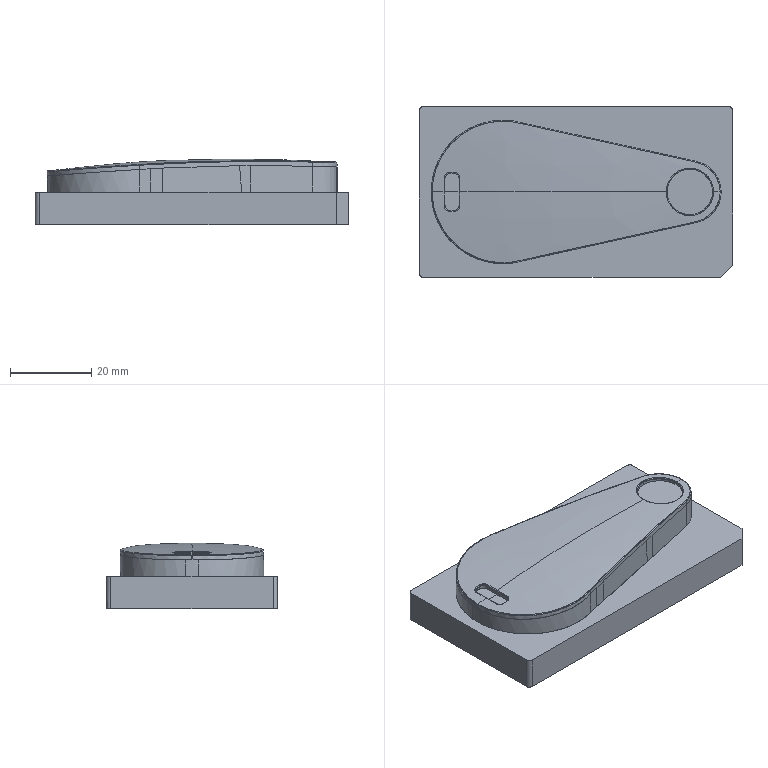NC program | PowerMill | posted with a generic post | part box 77 x 42 x 16.114 mm
Lines 17578 to 18293 of 134652:
N17675 M6
N17676 S18000 M03
N17677 G00 G90 X0.0 Y0.0
N17678 G43 Z10.803 H7
N17679
N17680 G05 P10000 R8
N17681 X35.0974 Y-6.155
N17682 Z-1.4614
N17683 G01 Z-2.6614 F1200.0
N17684 X35.0633 Y-6.1892 Z-2.6414 F2000.0
N17685 X35.0136 Y-6.2388 Z-2.6177
N17686 X34.9538 Y-6.2987 Z-2.5949
N17687 X34.8809 Y-6.3715 Z-2.5733
N17688 X34.7915 Y-6.4609 Z-2.5538
N17689 X34.711 Y-6.5414 Z-2.5419
N17690 X34.6456 Y-6.6069 Z-2.5361
N17691 X34.5916 Y-6.6609 Z-2.5342
N17692 X34.5388 Y-6.7136 Z-2.5355
N17693 X34.482 Y-6.7704 Z-2.5401
N17694 X34.388 Y-6.8644 Z-2.5527
N17695 X34.3036 Y-6.9488 Z-2.5709
N17696 X34.2267 Y-7.0258 Z-2.5946
N17697 X34.1559 Y-7.0966 Z-2.6239
N17698 X34.0903 Y-7.1621 Z-2.6586
N17699 X34.029 Y-7.2234 Z-2.6992
N17700 X33.6957 Y-7.4719 Z-2.6101
N17701 X33.7483 Y-7.4193 Z-2.5656
N17702 X33.8073 Y-7.3602 Z-2.5243
N17703 X33.8738 Y-7.2938 Z-2.4858
N17704 X33.9483 Y-7.2193 Z-2.4504
N17705 X34.0316 Y-7.136 Z-2.4185
N17706 X34.1246 Y-7.043 Z-2.3906
N17707 X34.2271 Y-6.9405 Z-2.3677
N17708 X34.3349 Y-6.8327 Z-2.3511
N17709 X34.4335 Y-6.734 Z-2.3421
N17710 X34.5208 Y-6.6468 Z-2.3389
N17711 X34.5972 Y-6.5704 Z-2.3399
N17712 X34.6638 Y-6.5038 Z-2.3437
N17713 X34.7235 Y-6.4441 Z-2.35
N17714 X34.8002 Y-6.3674 Z-2.3616
N17715 X34.8886 Y-6.2789 Z-2.379
N17716 X34.9883 Y-6.1793 Z-2.4046
N17717 X35.0858 Y-6.0818 Z-2.4365
N17718 X35.1732 Y-5.9944 Z-2.4723
N17719 X35.2506 Y-5.917 Z-2.5109
N17720 X35.3188 Y-5.8487 Z-2.552
N17721 X35.379 Y-5.7886 Z-2.5954
N17722 X35.4317 Y-5.7358 Z-2.6411
N17723 X35.4585 Y-5.7091 Z-2.6679
N17724 X35.7163 Y-5.3665 Z-2.7108
N17725 X35.6786 Y-5.4042 Z-2.6572
N17726 X35.6346 Y-5.4481 Z-2.6053
N17727 X35.5843 Y-5.4984 Z-2.5559
N17728 X35.5259 Y-5.5568 Z-2.5078
N17729 X35.4563 Y-5.6264 Z-2.4589
N17730 X35.3771 Y-5.7056 Z-2.41
N17731 X35.2948 Y-5.7879 Z-2.366
N17732 X35.2047 Y-5.8781 Z-2.3261
N17733 X35.1057 Y-5.9771 Z-2.2903
N17734 X34.9972 Y-6.0855 Z-2.2589
N17735 X34.8755 Y-6.2072 Z-2.2315
N17736 X34.7492 Y-6.3335 Z-2.2109
N17737 X34.6199 Y-6.4628 Z-2.1979
N17738 X34.4902 Y-6.5925 Z-2.1927
N17739 X34.3627 Y-6.7201 Z-2.1954
N17740 X34.2387 Y-6.844 Z-2.2056
N17741 X34.117 Y-6.9657 Z-2.2231
N17742 X34.0052 Y-7.0776 Z-2.2459
N17743 X33.9036 Y-7.1791 Z-2.2736
N17744 X33.8109 Y-7.2719 Z-2.3062
N17745 X33.7258 Y-7.3569 Z-2.3434
N17746 X33.6459 Y-7.4368 Z-2.3858
N17747 X33.5701 Y-7.5126 Z-2.4317
N17748 X33.507 Y-7.5757 Z-2.4765
N17749 X33.4525 Y-7.6302 Z-2.5228
N17750 X33.4042 Y-7.6786 Z-2.5719
N17751 X33.3589 Y-7.7238 Z-2.6266
N17752 X33.1083 Y-7.8896 Z-2.6082
N17753 X33.147 Y-7.8509 Z-2.5549
N17754 X33.193 Y-7.8049 Z-2.5017
N17755 X33.2475 Y-7.7504 Z-2.4482
N17756 X33.3114 Y-7.6865 Z-2.3945
N17757 X33.3847 Y-7.6131 Z-2.3416
N17758 X33.4591 Y-7.5388 Z-2.2955
N17759 X33.5247 Y-7.4732 Z-2.2602
N17760 X33.587 Y-7.4108 Z-2.2308
N17761 X33.6804 Y-7.3175 Z-2.1935
N17762 X33.7849 Y-7.2129 Z-2.1595
N17763 X33.9008 Y-7.0971 Z-2.1296
N17764 X34.0199 Y-6.978 Z-2.106
N17765 X34.1338 Y-6.864 Z-2.0894
N17766 X34.2679 Y-6.7299 Z-2.0772
N17767 X34.4058 Y-6.5921 Z-2.0725
N17768 X34.5458 Y-6.452 Z-2.0757
N17769 X34.6855 Y-6.3123 Z-2.0867
N17770 X34.8223 Y-6.1756 Z-2.1053
N17771 X34.9547 Y-6.0431 Z-2.131
N17772 X35.08 Y-5.9179 Z-2.1625
N17773 X35.1945 Y-5.8034 Z-2.1985
N17774 X35.3 Y-5.6979 Z-2.2391
N17775 X35.3979 Y-5.5999 Z-2.2843
N17776 X35.4892 Y-5.5087 Z-2.3342
N17777 X35.5745 Y-5.4234 Z-2.3888
N17778 X35.6349 Y-5.3629 Z-2.433
N17779 X35.7037 Y-5.2942 Z-2.4894
N17780 X35.7612 Y-5.2367 Z-2.544
N17781 X35.81 Y-5.1879 Z-2.5985
N17782 X35.8516 Y-5.1463 Z-2.6538
N17783 X35.8868 Y-5.111 Z-2.7106
N17784 X35.8915 Y-5.1063 Z-2.7191
N17785 X36.0308 Y-4.8822 Z-2.7188
N17786 X36.0101 Y-4.9029 Z-2.6799
N17787 X35.9738 Y-4.9392 Z-2.6207
N17788 X35.9313 Y-4.9818 Z-2.5626
N17789 X35.8814 Y-5.0316 Z-2.5052
N17790 X35.829 Y-5.084 Z-2.4525
N17791 X35.7752 Y-5.1378 Z-2.403
N17792 X35.7075 Y-5.2055 Z-2.3477
N17793 X35.6321 Y-5.2809 Z-2.295
N17794 X35.548 Y-5.365 Z-2.2448
N17795 X35.4534 Y-5.4597 Z-2.1966
N17796 X35.3456 Y-5.5674 Z-2.1495
N17797 X35.2307 Y-5.6823 Z-2.1061
N17798 X35.1114 Y-5.8016 Z-2.0686
N17799 X34.9828 Y-5.9303 Z-2.0361
N17800 X34.8437 Y-6.0694 Z-2.0088
N17801 X34.7232 Y-6.1898 Z-1.9908
N17802 X34.5989 Y-6.3142 Z-1.9778
N17803 X34.4641 Y-6.4489 Z-1.9702
N17804 X34.3204 Y-6.5926 Z-1.9691
N17805 X34.1721 Y-6.7409 Z-1.9756
N17806 X34.0288 Y-6.8842 Z-1.9895
N17807 X33.8939 Y-7.0191 Z-2.0099
N17808 X33.7684 Y-7.1446 Z-2.0359
N17809 X33.6524 Y-7.2606 Z-2.0666
N17810 X33.545 Y-7.368 Z-2.1017
N17811 X33.4385 Y-7.4745 Z-2.1433
N17812 X33.3435 Y-7.5696 Z-2.1876
N17813 X33.2574 Y-7.6556 Z-2.2351
N17814 X33.1789 Y-7.7342 Z-2.2862
N17815 X33.129 Y-7.784 Z-2.323
N17816 X33.062 Y-7.851 Z-2.3786
N17817 X33.0044 Y-7.9086 Z-2.4341
N17818 X32.9558 Y-7.9572 Z-2.489
N17819 X32.9153 Y-7.9977 Z-2.5436
N17820 X32.8819 Y-8.0311 Z-2.598
N17821 X32.6789 Y-8.1492 Z-2.5862
N17822 X32.714 Y-8.1142 Z-2.525
N17823 X32.7556 Y-8.0726 Z-2.4646
N17824 X32.8042 Y-8.0239 Z-2.405
N17825 X32.8603 Y-7.9679 Z-2.3465
N17826 X32.9241 Y-7.9041 Z-2.2895
N17827 X32.9948 Y-7.8334 Z-2.2353
N17828 X33.0457 Y-7.7825 Z-2.2009
N17829 X33.1387 Y-7.6894 Z-2.145
N17830 X33.2335 Y-7.5946 Z-2.0954
N17831 X33.3308 Y-7.4973 Z-2.052
N17832 X33.4394 Y-7.3888 Z-2.0116
N17833 X33.5423 Y-7.2858 Z-1.9796
N17834 X33.6483 Y-7.1798 Z-1.9518
N17835 X33.7747 Y-7.0535 Z-1.9253
N17836 X33.909 Y-6.9192 Z-1.9041
N17837 X34.055 Y-6.7732 Z-1.8884
N17838 X34.2107 Y-6.6175 Z-1.8793
N17839 X34.3664 Y-6.4618 Z-1.8779
N17840 X34.5119 Y-6.3162 Z-1.8833
N17841 X34.6451 Y-6.183 Z-1.8943
N17842 X34.7678 Y-6.0604 Z-1.9099
N17843 X34.9201 Y-5.9081 Z-1.9358
N17844 X35.0632 Y-5.7649 Z-1.9674
N17845 X35.1946 Y-5.6336 Z-2.0035
N17846 X35.3146 Y-5.5136 Z-2.0436
N17847 X35.4092 Y-5.419 Z-2.0809
N17848 X35.523 Y-5.3052 Z-2.1321
N17849 X35.6206 Y-5.2076 Z-2.1827
N17850 X35.7058 Y-5.1223 Z-2.234
N17851 X35.7812 Y-5.047 Z-2.2868
N17852 X35.8544 Y-4.9738 Z-2.3454
N17853 X35.9252 Y-4.903 Z-2.4089
N17854 X35.9862 Y-4.8419 Z-2.4715
N17855 X36.0387 Y-4.7894 Z-2.5339
N17856 X36.0838 Y-4.7444 Z-2.5967
N17857 X36.1222 Y-4.706 Z-2.6603
N17858 X36.1244 Y-4.7037 Z-2.6645
N17859 X36.1483 Y-4.6798 Z-2.7143
N17860 X36.2466 Y-4.4967 Z-2.6989
N17861 X36.2268 Y-4.5165 Z-2.6565
N17862 X36.1952 Y-4.5481 Z-2.6002
N17863 X36.1553 Y-4.588 Z-2.5401
N17864 X36.1057 Y-4.6376 Z-2.4756
N17865 X36.0452 Y-4.6981 Z-2.4069
N17866 X35.983 Y-4.7603 Z-2.3445
N17867 X35.9294 Y-4.8139 Z-2.2962
N17868 X35.884 Y-4.8593 Z-2.2589
N17869 X35.8419 Y-4.9014 Z-2.2276
N17870 X35.7958 Y-4.9475 Z-2.1961
N17871 X35.6958 Y-5.0475 Z-2.1342
N17872 X35.5896 Y-5.1537 Z-2.0771
N17873 X35.4768 Y-5.2665 Z-2.0246
N17874 X35.3562 Y-5.3871 Z-1.9769
N17875 X35.2267 Y-5.5166 Z-1.9336
N17876 X35.0865 Y-5.6568 Z-1.8946
N17877 X34.9358 Y-5.8075 Z-1.8606
N17878 X34.7806 Y-5.9628 Z-1.8336
N17879 X34.6206 Y-6.1227 Z-1.8137
N17880 X34.4555 Y-6.2878 Z-1.8011
N17881 X34.2851 Y-6.4582 Z-1.7959
N17882 X34.1205 Y-6.6228 Z-1.7985
N17883 X33.9617 Y-6.7816 Z-1.8086
N17884 X33.8082 Y-6.9351 Z-1.826
N17885 X33.6598 Y-7.0835 Z-1.8505
N17886 X33.516 Y-7.2273 Z-1.8819
N17887 X33.3765 Y-7.3668 Z-1.9202
N17888 X33.2587 Y-7.4846 Z-1.9594
N17889 X33.148 Y-7.5954 Z-2.0034
N17890 X33.0465 Y-7.6968 Z-2.0511
N17891 X32.9533 Y-7.79 Z-2.1025
N17892 X32.8677 Y-7.8756 Z-2.1576
N17893 X32.7889 Y-7.9544 Z-2.2164
N17894 X32.7145 Y-8.0288 Z-2.2803
N17895 X32.6514 Y-8.0919 Z-2.342
N17896 X32.5978 Y-8.1455 Z-2.4025
N17897 X32.552 Y-8.1913 Z-2.4631
N17898 X32.513 Y-8.2303 Z-2.5246
N17899 X32.4799 Y-8.2634 Z-2.5877
N17900 X32.3001 Y-8.3584 Z-2.584
N17901 X32.3304 Y-8.328 Z-2.5225
N17902 X32.368 Y-8.2905 Z-2.4594
N17903 X32.4135 Y-8.245 Z-2.3947
N17904 X32.4676 Y-8.1909 Z-2.3285
N17905 X32.5298 Y-8.1287 Z-2.2624
N17906 X32.5929 Y-8.0655 Z-2.2035
N17907 X32.6496 Y-8.0088 Z-2.1565
N17908 X32.6991 Y-7.9594 Z-2.1197
N17909 X32.7472 Y-7.9113 Z-2.0874
N17910 X32.8401 Y-7.8184 Z-2.0306
N17911 X32.9347 Y-7.7238 Z-1.9801
N17912 X33.0367 Y-7.6218 Z-1.9333
N17913 X33.1485 Y-7.5099 Z-1.8901
N17914 X33.2559 Y-7.4026 Z-1.855
N17915 X33.3587 Y-7.2997 Z-1.8257
N17916 X33.4938 Y-7.1647 Z-1.7933
N17917 X33.6312 Y-7.0272 Z-1.7676
N17918 X33.7809 Y-6.8775 Z-1.7467
N17919 X33.9428 Y-6.7157 Z-1.7317
N17920 X34.1137 Y-6.5448 Z-1.7237
N17921 X34.2796 Y-6.3789 Z-1.7231
N17922 X34.4329 Y-6.2256 Z-1.7288
N17923 X34.5747 Y-6.0838 Z-1.7395
N17924 X34.7229 Y-5.9356 Z-1.7563
N17925 X34.8799 Y-5.7785 Z-1.7807
N17926 X35.0358 Y-5.6227 Z-1.8122
N17927 X35.184 Y-5.4744 Z-1.8496
N17928 X35.3226 Y-5.3358 Z-1.892
N17929 X35.4514 Y-5.2071 Z-1.9388
N17930 X35.5707 Y-5.0878 Z-1.9894
N17931 X35.6811 Y-4.9773 Z-2.0435
N17932 X35.7849 Y-4.8736 Z-2.1019
N17933 X35.8779 Y-4.7805 Z-2.1618
N17934 X35.9617 Y-4.6968 Z-2.2234
N17935 X36.0373 Y-4.6212 Z-2.2871
N17936 X36.097 Y-4.5614 Z-2.3443
N17937 X36.1606 Y-4.4978 Z-2.4133
N17938 X36.2153 Y-4.4432 Z-2.4812
N17939 X36.2622 Y-4.3962 Z-2.5489
N17940 X36.3023 Y-4.3562 Z-2.6169
N17941 X36.336 Y-4.3224 Z-2.6857
N17942 X36.3398 Y-4.3187 Z-2.6943
N17943 X36.4252 Y-4.1484 Z-2.6965
N17944 X36.4205 Y-4.1531 Z-2.6848
N17945 X36.394 Y-4.1796 Z-2.6274
N17946 X36.3595 Y-4.2141 Z-2.565
N17947 X36.3155 Y-4.2581 Z-2.497
N17948 X36.2605 Y-4.3131 Z-2.423
N17949 X36.2052 Y-4.3684 Z-2.3567
N17950 X36.1582 Y-4.4154 Z-2.3055
N17951 X36.118 Y-4.4556 Z-2.265
N17952 X36.0768 Y-4.4968 Z-2.2267
N17953 X36.0345 Y-4.5391 Z-2.1917
N17954 X35.9468 Y-4.6268 Z-2.1274
N17955 X35.8494 Y-4.7242 Z-2.0643
N17956 X35.7406 Y-4.833 Z-2.0021
N17957 X35.6382 Y-4.9354 Z-1.9506
N17958 X35.5439 Y-5.0297 Z-1.9088
N17959 X35.4343 Y-5.1393 Z-1.8659
N17960 X35.2926 Y-5.281 Z-1.8175
N17961 X35.1442 Y-5.4294 Z-1.7748
N17962 X34.9978 Y-5.5759 Z-1.7406
N17963 X34.822 Y-5.7516 Z-1.7079
N17964 X34.6455 Y-5.9281 Z-1.683
N17965 X34.4673 Y-6.1063 Z-1.6659
N17966 X34.2871 Y-6.2865 Z-1.6566
N17967 X34.1049 Y-6.4687 Z-1.6552
N17968 X33.9558 Y-6.6178 Z-1.6598
N17969 X33.8068 Y-6.7668 Z-1.6701
N17970 X33.6581 Y-6.9155 Z-1.686
N17971 X33.5097 Y-7.0639 Z-1.7077
N17972 X33.3963 Y-7.1773 Z-1.7289
N17973 X33.2834 Y-7.2902 Z-1.755
N17974 X33.1579 Y-7.4157 Z-1.79
N17975 X33.0249 Y-7.5487 Z-1.8343
N17976 X32.9096 Y-7.6641 Z-1.8792
N17977 X32.8006 Y-7.773 Z-1.9283
N17978 X32.7101 Y-7.8635 Z-1.9751
N17979 X32.6165 Y-7.9571 Z-2.0308
N17980 X32.53 Y-8.0436 Z-2.0904
N17981 X32.4497 Y-8.1239 Z-2.1539
N17982 X32.411 Y-8.1626 Z-2.1879
N17983 X32.371 Y-8.2026 Z-2.2266
N17984 X32.3234 Y-8.2502 Z-2.2779
N17985 X32.2672 Y-8.3064 Z-2.3462
N17986 X32.219 Y-8.3546 Z-2.4127
N17987 X32.182 Y-8.3916 Z-2.471
N17988 X32.1539 Y-8.4197 Z-2.5226
N17989 X32.1314 Y-8.4422 Z-2.5727
N17990 X31.9654 Y-8.5234 Z-2.5734
N17991 X31.9995 Y-8.4893 Z-2.4979
N17992 X32.0386 Y-8.4502 Z-2.4259
N17993 X32.0833 Y-8.4054 Z-2.3562
N17994 X32.1341 Y-8.3546 Z-2.2887
N17995 X32.1915 Y-8.2972 Z-2.223
N17996 X32.2563 Y-8.2325 Z-2.1589
N17997 X32.3295 Y-8.1593 Z-2.0957
N17998 X32.4127 Y-8.0761 Z-2.0328
N17999 X32.5085 Y-7.9803 Z-1.9691
N18000 X32.6099 Y-7.8789 Z-1.9103
N18001 X32.7181 Y-7.7707 Z-1.856
N18002 X32.8336 Y-7.6551 Z-1.8063
N18003 X32.9575 Y-7.5313 Z-1.7611
N18004 X33.0907 Y-7.3981 Z-1.7205
N18005 X33.237 Y-7.2517 Z-1.6838
N18006 X33.3911 Y-7.0977 Z-1.6531
N18007 X33.5542 Y-6.9346 Z-1.6285
N18008 X33.7284 Y-6.7603 Z-1.6099
N18009 X33.8923 Y-6.5965 Z-1.5988
N18010 X34.0662 Y-6.4226 Z-1.5937
N18011 X34.2457 Y-6.2431 Z-1.5956
N18012 X34.4335 Y-6.0553 Z-1.6053
N18013 X34.6201 Y-5.8687 Z-1.6226
N18014 X34.7976 Y-5.6912 Z-1.6465
N18015 X34.9702 Y-5.5185 Z-1.677
N18016 X35.0715 Y-5.4173 Z-1.6984
N18017 X35.1772 Y-5.3116 Z-1.7244
N18018 X35.2957 Y-5.193 Z-1.7582
N18019 X35.4271 Y-5.0616 Z-1.8016
N18020 X35.5629 Y-4.9259 Z-1.8536
N18021 X35.6877 Y-4.8011 Z-1.9089
N18022 X35.7997 Y-4.689 Z-1.9656
N18023 X35.9 Y-4.5888 Z-2.0233
N18024 X35.9896 Y-4.4991 Z-2.0818
N18025 X36.0733 Y-4.4155 Z-2.1437
N18026 X36.1439 Y-4.3449 Z-2.2028
N18027 X36.2151 Y-4.2737 Z-2.2695
N18028 X36.2808 Y-4.208 Z-2.3394
N18029 X36.3394 Y-4.1493 Z-2.4106
N18030 X36.3908 Y-4.098 Z-2.4825
N18031 X36.4353 Y-4.0535 Z-2.5549
N18032 X36.4731 Y-4.0156 Z-2.6278
N18033 X36.5046 Y-3.9841 Z-2.7006
N18034 X36.5773 Y-3.8266 Z-2.7049
N18035 X36.577 Y-3.8269 Z-2.7041
N18036 X36.5438 Y-3.8601 Z-2.625
N18037 X36.5049 Y-3.899 Z-2.5476
N18038 X36.46 Y-3.9439 Z-2.4719
N18039 X36.4092 Y-3.9947 Z-2.3983
N18040 X36.3524 Y-4.0515 Z-2.3273
N18041 X36.29 Y-4.1139 Z-2.2592
N18042 X36.2156 Y-4.1883 Z-2.1873
N18043 X36.1344 Y-4.2695 Z-2.1183
N18044 X36.0456 Y-4.3583 Z-2.0519
N18045 X35.9479 Y-4.456 Z-1.9875
N18046 X35.8449 Y-4.559 Z-1.9275
N18047 X35.733 Y-4.6709 Z-1.8701
N18048 X35.616 Y-4.7879 Z-1.8176
N18049 X35.4883 Y-4.9156 Z-1.7677
N18050 X35.349 Y-5.0549 Z-1.7207
N18051 X35.1971 Y-5.2068 Z-1.6772
N18052 X35.0328 Y-5.3711 Z-1.6379
N18053 X34.8599 Y-5.544 Z-1.6044
N18054 X34.695 Y-5.7089 Z-1.5792
N18055 X34.5437 Y-5.8602 Z-1.5615
N18056 X34.4065 Y-5.9974 Z-1.5497
N18057 X34.2337 Y-6.1702 Z-1.5405
N18058 X34.0398 Y-6.3641 Z-1.5371
N18059 X33.8484 Y-6.5555 Z-1.5412
N18060 X33.6647 Y-6.7392 Z-1.5525
N18061 X33.4922 Y-6.9117 Z-1.5702
N18062 X33.3183 Y-7.0856 Z-1.5957
N18063 X33.1593 Y-7.2446 Z-1.6261
N18064 X33.012 Y-7.3919 Z-1.6613
N18065 X32.8745 Y-7.5294 Z-1.7014
N18066 X32.7452 Y-7.6587 Z-1.7466
N18067 X32.6228 Y-7.7811 Z-1.7972
N18068 X32.5062 Y-7.8977 Z-1.8531
N18069 X32.4137 Y-7.9902 Z-1.9036
N18070 X32.3228 Y-8.0811 Z-1.961
N18071 X32.2326 Y-8.1713 Z-2.0265
N18072 X32.1436 Y-8.2603 Z-2.1001
N18073 X32.0893 Y-8.3146 Z-2.1496
N18074 X32.0371 Y-8.3668 Z-2.2032
N18075 X31.9839 Y-8.42 Z-2.2663
N18076 X31.9362 Y-8.4677 Z-2.3308
N18077 X31.8995 Y-8.5044 Z-2.3872
N18078 X31.8601 Y-8.5438 Z-2.456
N18079 X31.8305 Y-8.5734 Z-2.5173
N18080 X31.8081 Y-8.5958 Z-2.5755
N18081 X31.6548 Y-8.6643 Z-2.5796
N18082 X31.6704 Y-8.6487 Z-2.5334
N18083 X31.6912 Y-8.6279 Z-2.4848
N18084 X31.7197 Y-8.5994 Z-2.4285
N18085 X31.7582 Y-8.5609 Z-2.3621
N18086 X31.8091 Y-8.51 Z-2.2851
N18087 X31.8518 Y-8.4672 Z-2.2277
N18088 X31.8875 Y-8.4315 Z-2.1846
N18089 X31.9195 Y-8.3995 Z-2.1498
N18090 X31.9904 Y-8.3287 Z-2.0807
N18091 X32.0683 Y-8.2507 Z-2.0141
N18092 X32.1547 Y-8.1644 Z-1.9493
N18093 X32.2423 Y-8.0767 Z-1.891
N18094 X32.3359 Y-7.9831 Z-1.8362
N18095 X32.4315 Y-7.8875 Z-1.7873
N18096 X32.5405 Y-7.7785 Z-1.7383
N18097 X32.6651 Y-7.6539 Z-1.6897
N18098 X32.8049 Y-7.5142 Z-1.643
N18099 X32.9351 Y-7.384 Z-1.6061
N18100 X33.0492 Y-7.2698 Z-1.5787
N18101 X33.1497 Y-7.1694 Z-1.5584
N18102 X33.3174 Y-7.0016 Z-1.5314
N18103 X33.4857 Y-6.8334 Z-1.511
N18104 X33.6543 Y-6.6648 Z-1.4964
N18105 X33.823 Y-6.496 Z-1.4878
N18106 X34.0163 Y-6.3027 Z-1.4848
N18107 X34.2166 Y-6.1024 Z-1.4891
N18108 X34.4187 Y-5.9003 Z-1.5012
N18109 X34.6161 Y-5.703 Z-1.5207
N18110 X34.8058 Y-5.5132 Z-1.5471
N18111 X34.9864 Y-5.3326 Z-1.5795
N18112 X35.1372 Y-5.1818 Z-1.6125
N18113 X35.273 Y-5.0461 Z-1.6476
N18114 X35.4198 Y-4.8993 Z-1.6923
N18115 X35.5631 Y-4.7559 Z-1.7434
N18116 X35.6948 Y-4.6243 Z-1.7976
N18117 X35.8139 Y-4.5052 Z-1.8538
N18118 X35.9199 Y-4.3991 Z-1.9106
N18119 X36.0246 Y-4.2945 Z-1.9741
N18120 X36.1198 Y-4.1992 Z-2.0396
N18121 X36.2071 Y-4.1119 Z-2.1078
N18122 X36.2873 Y-4.0318 Z-2.1788
N18123 X36.361 Y-3.958 Z-2.253
N18124 X36.4241 Y-3.8949 Z-2.3249
N18125 X36.4803 Y-3.8388 Z-2.3979
N18126 X36.5295 Y-3.7896 Z-2.4719
N18127 X36.5721 Y-3.7469 Z-2.5466
N18128 X36.6084 Y-3.7106 Z-2.6221
N18129 X36.6371 Y-3.6819 Z-2.6938
N18130 X36.702 Y-3.5322 Z-2.7063
N18131 X36.6809 Y-3.5533 Z-2.6502
N18132 X36.6454 Y-3.5888 Z-2.5696
N18133 X36.6043 Y-3.6299 Z-2.4911
N18134 X36.5573 Y-3.6769 Z-2.4146
N18135 X36.5042 Y-3.73 Z-2.3398
N18136 X36.4443 Y-3.7899 Z-2.2665
N18137 X36.377 Y-3.8572 Z-2.1943
N18138 X36.3012 Y-3.933 Z-2.1228
N18139 X36.2157 Y-4.0185 Z-2.0511
N18140 X36.1215 Y-4.1127 Z-1.9805
N18141 X36.025 Y-4.2092 Z-1.9164
N18142 X35.9209 Y-4.3133 Z-1.8557
N18143 X35.8079 Y-4.4263 Z-1.798
N18144 X35.6872 Y-4.547 Z-1.7442
N18145 X35.5645 Y-4.6697 Z-1.6957
N18146 X35.4217 Y-4.8125 Z-1.6463
N18147 X35.273 Y-4.9612 Z-1.6022
N18148 X35.1123 Y-5.1219 Z-1.5617
N18149 X34.9388 Y-5.2954 Z-1.5255
N18150 X34.7524 Y-5.4818 Z-1.4942
N18151 X34.5552 Y-5.679 Z-1.469
N18152 X34.357 Y-5.8772 Z-1.4512
N18153 X34.1705 Y-6.0637 Z-1.4408
N18154 X33.9984 Y-6.2357 Z-1.4366
N18155 X33.8362 Y-6.398 Z-1.4373
N18156 X33.6627 Y-6.5714 Z-1.4433
N18157 X33.474 Y-6.7602 Z-1.4564
N18158 X33.2867 Y-6.9474 Z-1.4765
N18159 X33.1136 Y-7.1206 Z-1.5023
N18160 X32.9556 Y-7.2786 Z-1.5327
N18161 X32.8103 Y-7.4239 Z-1.5671
N18162 X32.699 Y-7.5352 Z-1.5985
N18163 X32.5882 Y-7.646 Z-1.6337
N18164 X32.4781 Y-7.7561 Z-1.6735
N18165 X32.3662 Y-7.868 Z-1.7205
N18166 X32.2589 Y-7.9753 Z-1.7726
N18167 X32.171 Y-8.0632 Z-1.8209
N18168 X32.0739 Y-8.1602 Z-1.8811
N18169 X31.9839 Y-8.2503 Z-1.9451
N18170 X31.9002 Y-8.334 Z-2.013
N18171 X31.8226 Y-8.4116 Z-2.0846
N18172 X31.7507 Y-8.4835 Z-2.16
N18173 X31.7218 Y-8.5124 Z-2.1936
N18174 X31.6891 Y-8.5451 Z-2.2359
N18175 X31.6498 Y-8.5844 Z-2.2925
N18176 X31.6021 Y-8.6321 Z-2.3697
N18177 X31.5656 Y-8.6686 Z-2.4368
N18178 X31.5391 Y-8.6951 Z-2.4926
N18179 X31.5199 Y-8.7143 Z-2.54
N18180 X31.5057 Y-8.7285 Z-2.5851
N18181 X31.358 Y-8.7914 Z-2.6042
N18182 X31.3631 Y-8.7862 Z-2.585
N18183 X31.3916 Y-8.7577 Z-2.5056
N18184 X31.4257 Y-8.7236 Z-2.4276
N18185 X31.4657 Y-8.6837 Z-2.3511
N18186 X31.5118 Y-8.6376 Z-2.276
N18187 X31.5642 Y-8.5851 Z-2.2024
N18188 X31.6233 Y-8.5261 Z-2.1305
N18189 X31.6891 Y-8.4603 Z-2.0605
N18190 X31.7613 Y-8.388 Z-1.9932
N18191 X31.8383 Y-8.3111 Z-1.9296
N18192 X31.9254 Y-8.224 Z-1.8651
N18193 X32.0148 Y-8.1346 Z-1.8066
N18194 X32.1129 Y-8.0364 Z-1.7505
N18195 X32.2208 Y-7.9286 Z-1.6971
N18196 X32.3286 Y-7.8208 Z-1.6504
N18197 X32.4354 Y-7.7139 Z-1.609
N18198 X32.5648 Y-7.5845 Z-1.5657
N18199 X32.7074 Y-7.4419 Z-1.5256
N18200 X32.8644 Y-7.285 Z-1.4893
N18201 X33.0331 Y-7.1163 Z-1.4578
N18202 X33.1817 Y-6.9677 Z-1.4356
N18203 X33.3598 Y-6.7895 Z-1.4156
N18204 X33.5396 Y-6.6097 Z-1.402
N18205 X33.7383 Y-6.411 Z-1.3937
N18206 X33.9541 Y-6.1952 Z-1.3923
N18207 X34.164 Y-5.9853 Z-1.3981
N18208 X34.3544 Y-5.7949 Z-1.4095
N18209 X34.5329 Y-5.6165 Z-1.4256
N18210 X34.7084 Y-5.4409 Z-1.4469
N18211 X34.8835 Y-5.2658 Z-1.4745
N18212 X35.0704 Y-5.0789 Z-1.511
N18213 X35.2442 Y-4.9052 Z-1.5521
N18214 X35.3765 Y-4.7728 Z-1.5885
N18215 X35.5136 Y-4.6357 Z-1.6323
N18216 X35.6538 Y-4.4956 Z-1.6841
N18217 X35.7869 Y-4.3625 Z-1.7409
N18218 X35.9103 Y-4.239 Z-1.8011
N18219 X36.0237 Y-4.1256 Z-1.864
N18220 X36.1276 Y-4.0217 Z-1.9292
N18221 X36.2155 Y-3.9338 Z-1.9912
N18222 X36.3036 Y-3.8458 Z-2.0608
N18223 X36.3827 Y-3.7667 Z-2.1316
N18224 X36.4538 Y-3.6956 Z-2.2036
N18225 X36.5176 Y-3.6318 Z-2.2773
N18226 X36.5757 Y-3.5737 Z-2.354
N18227 X36.6283 Y-3.5211 Z-2.4332
N18228 X36.6733 Y-3.4761 Z-2.5114
N18229 X36.7113 Y-3.438 Z-2.589
N18230 X36.7429 Y-3.4064 Z-2.6663
N18231 X36.7672 Y-3.3822 Z-2.7392
N18232 X36.8157 Y-3.2488 Z-2.7329
N18233 X36.7996 Y-3.2649 Z-2.6823
N18234 X36.7687 Y-3.2958 Z-2.6008
N18235 X36.7328 Y-3.3317 Z-2.522
N18236 X36.6943 Y-3.3702 Z-2.4512
N18237 X36.6404 Y-3.4241 Z-2.3663
N18238 X36.5812 Y-3.4833 Z-2.2847
N18239 X36.5161 Y-3.5483 Z-2.206
N18240 X36.4449 Y-3.6195 Z-2.1303
N18241 X36.3672 Y-3.6973 Z-2.0573
N18242 X36.2822 Y-3.7823 Z-1.9869
N18243 X36.1894 Y-3.8751 Z-1.9189
N18244 X36.0877 Y-3.9768 Z-1.8532
N18245 X35.9759 Y-4.0886 Z-1.7894
N18246 X35.854 Y-4.2105 Z-1.7279
N18247 X35.723 Y-4.3415 Z-1.6699
N18248 X35.5823 Y-4.4822 Z-1.6155
N18249 X35.4313 Y-4.6332 Z-1.5651
N18250 X35.2695 Y-4.795 Z-1.5191
N18251 X35.0977 Y-4.9668 Z-1.4782
N18252 X34.9194 Y-5.1451 Z-1.4431
N18253 X34.7429 Y-5.3216 Z-1.415
N18254 X34.523 Y-5.5415 Z-1.3872
N18255 X34.3021 Y-5.7624 Z-1.3672
N18256 X34.0791 Y-5.9854 Z-1.355
N18257 X33.8543 Y-6.2102 Z-1.3507
N18258 X33.6291 Y-6.4354 Z-1.3542
N18259 X33.4121 Y-6.6523 Z-1.3646
N18260 X33.2131 Y-6.8513 Z-1.3812
N18261 X33.0277 Y-7.0368 Z-1.4039
N18262 X32.8529 Y-7.2115 Z-1.4326
N18263 X32.6871 Y-7.3774 Z-1.4673
N18264 X32.5288 Y-7.5357 Z-1.5081
N18265 X32.377 Y-7.6875 Z-1.5548
N18266 X32.2474 Y-7.8171 Z-1.6014
N18267 X32.1263 Y-7.9382 Z-1.6523
N18268 X32.0129 Y-8.0515 Z-1.7076
N18269 X31.9068 Y-8.1577 Z-1.7673
N18270 X31.8072 Y-8.2573 Z-1.8313
N18271 X31.7138 Y-8.3507 Z-1.8996
N18272 X31.6337 Y-8.4308 Z-1.966
N18273 X31.5611 Y-8.5034 Z-2.0345
N18274 X31.4956 Y-8.5689 Z-2.105
N18275 X31.437 Y-8.6275 Z-2.1774
N18276 X31.3847 Y-8.6797 Z-2.2517
N18277 X31.3453 Y-8.7192 Z-2.3154
N18278 X31.3034 Y-8.7611 Z-2.3921
N18279 X31.2691 Y-8.7953 Z-2.4664
N18280 X31.2416 Y-8.8229 Z-2.5392
N18281 X31.2201 Y-8.8444 Z-2.6114
N18282 X31.0923 Y-8.8873 Z-2.5921
N18283 X31.1124 Y-8.8672 Z-2.525
N18284 X31.1389 Y-8.8407 Z-2.4549
N18285 X31.1729 Y-8.8068 Z-2.3801
N18286 X31.215 Y-8.7647 Z-2.301
N18287 X31.2648 Y-8.7149 Z-2.2202
N18288 X31.3166 Y-8.663 Z-2.147
N18289 X31.3658 Y-8.6138 Z-2.0862
N18290 X31.4148 Y-8.5648 Z-2.0325
N18291 X31.4894 Y-8.4902 Z-1.9595
N18292 X31.5706 Y-8.4091 Z-1.8895
N18293 X31.6588 Y-8.3208 Z-1.8225
N18294 X31.7549 Y-8.2248 Z-1.7584
N18295 X31.8596 Y-8.1201 Z-1.6971
N18296 X31.9577 Y-8.0219 Z-1.6463
N18297 X32.066 Y-7.9137 Z-1.5972
N18298 X32.1754 Y-7.8042 Z-1.554
N18299 X32.2961 Y-7.6835 Z-1.5122
N18300 X32.4409 Y-7.5387 Z-1.4688
N18301 X32.5883 Y-7.3913 Z-1.4312
N18302 X32.7116 Y-7.268 Z-1.4044
N18303 X32.8245 Y-7.1552 Z-1.3837
N18304 X32.9376 Y-7.042 Z-1.3667
N18305 X33.1385 Y-6.8411 Z-1.3428
N18306 X33.3466 Y-6.633 Z-1.3256
N18307 X33.566 Y-6.4136 Z-1.3151
N18308 X33.7946 Y-6.1851 Z-1.3121
N18309 X34.0271 Y-5.9526 Z-1.3167
N18310 X34.2517 Y-5.7279 Z-1.3285
N18311 X34.4513 Y-5.5283 Z-1.3447
N18312 X34.6506 Y-5.329 Z-1.367
N18313 X34.8495 Y-5.1302 Z-1.3962
N18314 X35.0477 Y-4.9319 Z-1.4328
N18315 X35.202 Y-4.7776 Z-1.4664
N18316 X35.3649 Y-4.6147 Z-1.5083
N18317 X35.5215 Y-4.4582 Z-1.5559
N18318 X35.6687 Y-4.3109 Z-1.6081
N18319 X35.806 Y-4.1737 Z-1.6643
N18320 X35.9336 Y-4.0461 Z-1.7241
N18321 X36.0521 Y-3.9275 Z-1.7872
N18322 X36.1627 Y-3.8169 Z-1.8539
N18323 X36.2621 Y-3.7175 Z-1.9216
N18324 X36.3527 Y-3.627 Z-1.9912
N18325 X36.4354 Y-3.5442 Z-2.0631
N18326 X36.511 Y-3.4687 Z-2.1375
N18327 X36.5799 Y-3.3997 Z-2.2144
N18328 X36.6427 Y-3.3369 Z-2.2941
N18329 X36.6997 Y-3.2799 Z-2.3766
N18330 X36.7418 Y-3.2378 Z-2.4455
N18331 X36.7816 Y-3.1981 Z-2.521
N18332 X36.8169 Y-3.1628 Z-2.6006
N18333 X36.8456 Y-3.134 Z-2.6793
N18334 X36.8597 Y-3.12 Z-2.7253
N18335 X36.9017 Y-2.993 Z-2.7185
N18336 X36.8886 Y-3.0062 Z-2.6735
N18337 X36.8629 Y-3.0318 Z-2.6021
N18338 X36.8297 Y-3.0651 Z-2.5259
N18339 X36.7882 Y-3.1066 Z-2.4451
N18340 X36.7395 Y-3.1553 Z-2.3629
N18341 X36.6934 Y-3.2014 Z-2.2941
N18342 X36.6523 Y-3.2425 Z-2.2387
N18343 X36.6119 Y-3.2829 Z-2.1894
N18344 X36.5449 Y-3.3499 Z-2.1161
N18345 X36.4645 Y-3.4303 Z-2.0373
N18346 X36.3788 Y-3.516 Z-1.963
N18347 X36.2878 Y-3.607 Z-1.8933
N18348 X36.1913 Y-3.7034 Z-1.8281
N18349 X36.081 Y-3.8138 Z-1.7617
N18350 X35.962 Y-3.9328 Z-1.6985
N18351 X35.8337 Y-4.0611 Z-1.6384
N18352 X35.6954 Y-4.1994 Z-1.5819
N18353 X35.547 Y-4.3478 Z-1.5293
N18354 X35.3897 Y-4.5051 Z-1.4813
N18355 X35.2277 Y-4.667 Z-1.4392
N18356 X35.0364 Y-4.8584 Z-1.3975
N18357 X34.836 Y-5.0588 Z-1.3616
N18358 X34.625 Y-5.2698 Z-1.3317
N18359 X34.4014 Y-5.4934 Z-1.3079
N18360 X34.2081 Y-5.6867 Z-1.2929
N18361 X34.0093 Y-5.8855 Z-1.2826
N18362 X33.7888 Y-6.106 Z-1.2772
N18363 X33.5493 Y-6.3454 Z-1.2785
N18364 X33.3272 Y-6.5676 Z-1.2868
N18365 X33.1266 Y-6.7682 Z-1.3008
N18366 X32.9283 Y-6.9665 Z-1.3213
N18367 X32.8041 Y-7.0907 Z-1.338
N18368 X32.6734 Y-7.2214 Z-1.3595
N18369 X32.526 Y-7.3687 Z-1.389
N18370 X32.364 Y-7.5308 Z-1.4283
N18371 X32.2125 Y-7.6823 Z-1.4722
N18372 X32.0771 Y-7.8176 Z-1.5183
N18373 X31.9565 Y-7.9383 Z-1.5657
N18374 X31.8436 Y-8.0511 Z-1.6167
N18375 X31.7441 Y-8.1507 Z-1.668
N18376 X31.6418 Y-8.253 Z-1.7274
N18377 X31.5486 Y-8.3462 Z-1.7893
N18378 X31.4634 Y-8.4314 Z-1.8538
N18379 X31.3821 Y-8.5127 Z-1.9236
N18380 X31.3208 Y-8.574 Z-1.9822
N18381 X31.2595 Y-8.6353 Z-2.0476
N18382 X31.1975 Y-8.6972 Z-2.1227
N18383 X31.1412 Y-8.7535 Z-2.2007
N18384 X31.0923 Y-8.8025 Z-2.2786
N18385 X31.0508 Y-8.844 Z-2.3553
N18386 X31.0166 Y-8.8781 Z-2.43
N18387 X30.9893 Y-8.9055 Z-2.5028
N18388 X30.9684 Y-8.9264 Z-2.5734
N18389 X30.8444 Y-8.9655 Z-2.5596
N18390 X30.8697 Y-8.9403 Z-2.4797